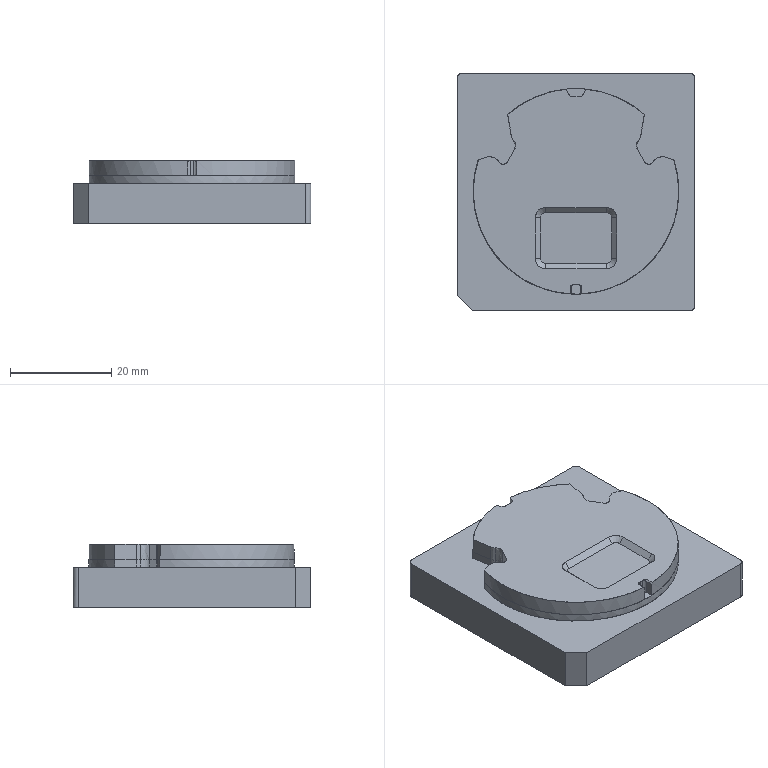NC program | PowerMill | posted with a generic post | part box 47 x 47 x 12.511 mm
Lines 16282 to 17389 of 232111:
N16379 M6
N16380 S8500 M03
N16381 G00 G90 X0.0 Y0.0
N16382 G43 Z11.801 H3
N16383
N16384 G05 P10000 R8
N16385 X-1.9559 Y31.1287
N16386 Z-2.08
N16387 G01 Z-3.28 F360.0
N16388 X-1.5441 Y25.8698 F600.0
N16389 G03 X-1.1674 Y25.6718 I0.4494 J0.3976
N16390 G01 X-0.8465 Y25.6171
N16391 X-0.5643 Y25.5515
N16392 X-0.2822 Y25.4696
N16393 X-0.199 Y25.4403
N16394 G03 X0.199 I0.199 J0.5661
N16395 G01 X0.2822 Y25.4696
N16396 X0.5643 Y25.5515
N16397 X0.8465 Y25.6171
N16398 X1.1287 Y25.6671
N16399 X1.4108 Y25.7015
N16400 X1.693 Y25.7211
N16401 X1.9523 Y25.7257
N16402 G03 X2.2593 Y25.8166 I-0.0106 J0.5999
N16403 G00 Z4.0015
N16404 G01 X7.284 Y30.297 F10000.0
N16405 G00 Z0.9315
N16406 G01 Z-0.2685 F360.0
N16407 X6.0222 Y25.1751 F600.0
N16408 X-18.9848 Y15.2852
N16409 X-18.9833 Y15.0806
N16410 X-18.966 Y14.793
N16411 X-18.9344 Y14.5106
N16412 X-18.9091 Y14.3457
N16413 X-18.5491 Y12.3094
N16414 X-18.8343 Y12.2512
N16415 X-19.2161 Y12.1568
N16416 X-19.495 Y12.0725
N16417 X-19.8583 Y11.9493
N16418 X-21.199 Y11.4604
N16419 X-21.3814 Y11.3897
N16420 X-21.5617 Y11.3136
N16421 X-21.7594 Y11.2206
N16422 X-22.0334 Y11.0742
N16423 X-22.1755 Y10.9915
N16424 X-22.3485 Y10.8815
N16425 X-22.6744 Y10.6481
N16426 X-22.9228 Y10.4449
N16427 X-23.1181 Y10.2662
N16428 X-23.3136 Y10.0694
N16429 X-23.4971 Y9.8645
N16430 X-23.6481 Y9.6794
N16431 X-23.7839 Y9.4976
N16432 X-23.948 Y9.2535
N16433 X-24.0661 Y9.0599
N16434 X-24.1824 Y8.8472
N16435 X-24.2906 Y8.6302
N16436 X-24.4151 Y8.3425
N16437 X-24.5201 Y8.0569
N16438 X12.4545 Y22.6798
N16439 X12.7482 Y22.5176
N16440 X13.3123 Y22.1867
N16441 X14.0252 Y21.7406
N16442 X14.5398 Y21.3978
N16443 X15.0415 Y21.0461
N16444 X15.5786 Y20.6499
N16445 X16.1484 Y20.2049
N16446 X16.5964 Y19.8366
N16447 X17.0379 Y19.4533
N16448 X-25.6557 Y2.5685
N16449 X-25.6952 Y2.1165
N16450 X-25.7221 Y1.7438
N16451 X-25.7538 Y1.1091
N16452 G03 X-25.7718 Y-0.1894 I32.4439 J-1.0979
N16453 G01 X-25.7592 Y-0.7348
N16454 X-25.7264 Y-1.4301
N16455 X-25.6889 Y-1.9481
N16456 X-25.6423 Y-2.4653
N16457 X18.9842 Y15.1839
N16458 X18.9835 Y15.0859
N16459 G02 X18.9091 Y14.3457 I-5.9029 J0.2194
N16460 G01 X18.549 Y12.3091
N16461 X18.75 Y12.2698
N16462 X19.2161 Y12.1568
N16463 X19.4948 Y12.0726
N16464 X19.8555 Y11.9502
N16465 X21.1965 Y11.4614
N16466 X21.3786 Y11.3908
N16467 X21.5624 Y11.3135
N16468 X21.7342 Y11.2323
N16469 X-24.7296 Y-7.1435
N16470 X-24.5357 Y-7.7749
N16471 X-24.279 Y-8.5315
N16472 X-24.0808 Y-9.07
N16473 X-23.8388 Y-9.6817
N16474 X-23.5679 Y-10.3164
N16475 X-23.293 Y-10.9154
N16476 X-23.0058 Y-11.501
N16477 X24.7274 Y7.3769
N16478 X24.7977 Y7.1419
N16479 X24.9346 Y6.6395
N16480 X25.0763 Y6.0727
N16481 X25.2312 Y5.3792
N16482 X25.3226 Y4.9198
N16483 X25.3803 Y4.602
N16484 X25.4836 Y3.9679
N16485 X25.5726 Y3.3334
N16486 X25.6438 Y2.7001
N16487 X-20.473 Y-15.5385
N16488 X-20.1109 Y-16.0027
N16489 X-19.8166 Y-16.361
N16490 X-19.5181 Y-16.7156
N16491 X-19.2019 Y-17.0755
N16492 X-19.0013 Y-17.2971
N16493 X-18.7087 Y-17.6101
N16494 X-18.2485 Y-18.0837
N16495 X-17.8897 Y-18.4363
N16496 X-17.5949 Y-18.7165
N16497 X-17.2957 Y-18.9919
N16498 X-17.0377 Y-19.219
N16499 X25.6558 Y-2.3343
N16500 X25.5832 Y-3.0141
N16501 X25.4974 Y-3.6491
N16502 X25.3955 Y-4.2838
N16503 X25.2768 Y-4.9186
N16504 X25.1764 Y-5.3914
N16505 X25.0694 Y-5.8627
N16506 X24.9355 Y-6.403
N16507 X24.7306 Y-7.1402
N16508 X24.5177 Y-7.8236
N16509 X-12.4535 Y-22.4452
N16510 X-12.2179 Y-22.5761
N16511 X-11.6955 Y-22.8502
N16512 X-11.0463 Y-23.169
N16513 X-10.5089 Y-23.4172
N16514 X-9.9513 Y-23.6579
N16515 X-9.3471 Y-23.9017
N16516 X-8.9157 Y-24.0648
N16517 X-8.3099 Y-24.2802
N16518 X-7.775 Y-24.4554
N16519 X-7.3136 Y-24.5975
N16520 X-6.8223 Y-24.7369
N16521 X-6.0249 Y-24.942
N16522 X21.5338 Y-14.0429
N16523 G00 Z11.801
N16524 G05 P0
N16525 (---------------)
N16526 ( END TOOLPATH : 精公基准台01-平坦面平行-D10 )
N16527 (---------------)
N16528 ( START TOOLPATH : 精公基准台01-基准面偏置-D10 )
N16529 (---------------)
N16530 G00 X0.0 Y0.0 Z9.8015
N16531 G05 P10000 R8
N16532 X-0.6019 Y34.255
N16533 Z-3.51
N16534 G01 Z-4.71 F360.0
N16535 Y28.98 F600.0
N16536 X-0.5663 Y25.8112
N16537 X0.0 Y25.8175
N16538 X0.5663 Y25.8112
N16539 G02 X2.2654 Y25.7174 I-0.551 J-25.4305
N16540 G01 X2.8317 Y25.661
N16541 X3.3981 Y25.5919
N16542 X4.1157 Y25.4857
N16543 X4.5308 Y25.4152
N16544 X5.0971 Y25.307
N16545 X5.6635 Y25.1856
N16546 X6.2298 Y25.051
N16547 X6.7962 Y24.9027
N16548 X7.3625 Y24.7404
N16549 X7.9289 Y24.564
N16550 X8.4952 Y24.3729
N16551 X9.0616 Y24.1671
N16552 X9.6279 Y23.9459
N16553 X10.1943 Y23.7092
N16554 X10.7606 Y23.4562
N16555 X11.327 Y23.1868
N16556 X11.8933 Y22.9
N16557 X12.4597 Y22.5953
N16558 X13.026 Y22.2718
N16559 X13.5924 Y21.9288
N16560 X14.2256 Y21.5212
N16561 X14.7251 Y21.1808
N16562 X15.2914 Y20.7735
N16563 X15.8578 Y20.3418
N16564 X16.499 Y19.8222
N16565 X17.1525 Y19.2558
N16566 X17.3869 Y19.0298
N16567 X17.5568 Y18.8471
N16568 X17.6915 Y18.6895
N16569 X17.9089 Y18.4063
N16570 X18.0723 Y18.1622
N16571 X22.1193 Y20.7449
N16572 G03 X20.6796 Y22.5214 I-8.5455 J-5.4534
N16573 G01 X20.0339 Y23.1489
N16574 G02 X20.4552 Y24.1693 I0.413 J0.4266
N16575 G01 X21.6227 Y24.1529
N16576 G02 X24.1544 Y21.597 I-0.0359 J-2.5674
N16577 G01 X24.1687 Y18.3761
N16578 G02 X23.2908 Y18.2225 I-0.452 J-0.002
N16579 G01 X23.1242 Y18.6908
N16580 G03 X22.1193 Y20.7449 I-9.5502 J-3.3993
N16581 G01 X18.0723 Y18.1622
N16582 X18.1231 Y18.0833
N16583 X18.2901 Y17.7907
N16584 X18.4066 Y17.5568
N16585 X18.5297 Y17.2736
N16586 X18.6339 Y16.9904
N16587 X18.6895 Y16.8151
N16588 X18.7907 Y16.4241
N16589 X18.8448 Y16.1409
N16590 X18.8833 Y15.8578
N16591 X18.9067 Y15.5746
N16592 X18.9151 Y15.2914
N16593 X18.9088 Y15.0082
N16594 X18.8872 Y14.7251
N16595 X18.8507 Y14.4419
N16596 X18.6281 Y13.1786
N16597 G03 X19.3043 Y12.0532 I0.9847 J-0.1742
N16598 G01 X19.7973 Y11.8933
N16599 X21.3431 Y11.327
N16600 X21.5212 Y11.2523
N16601 X21.8044 Y11.1174
N16602 X22.0876 Y10.9608
N16603 X22.4003 Y10.7606
N16604 X22.6539 Y10.5748
N16605 X22.851 Y10.4138
N16606 X23.0914 Y10.1943
N16607 X23.2203 Y10.0651
N16608 X23.4385 Y9.8247
N16609 X23.5986 Y9.6279
N16610 X23.7866 Y9.3699
N16611 X23.9827 Y9.0616
N16612 X24.1381 Y8.7784
N16613 X24.2725 Y8.4952
N16614 X24.353 Y8.3019
N16615 X24.4843 Y7.9289
N16616 X24.658 Y7.3625
N16617 X24.8176 Y6.7962
N16618 X24.963 Y6.2298
N16619 X25.0949 Y5.6635
N16620 X25.2133 Y5.0971
N16621 X25.3184 Y4.5308
N16622 X25.4107 Y3.9644
N16623 X25.4901 Y3.3981
N16624 X25.5567 Y2.8317
N16625 X25.6107 Y2.2654
N16626 X25.6519 Y1.699
N16627 X25.6804 Y1.1327
N16628 X25.6961 Y0.5663
N16629 X25.7003 Y0.0
N16630 X25.6914 Y-0.5663
N16631 X25.6701 Y-1.1327
N16632 X25.6361 Y-1.699
N16633 X25.5899 Y-2.2654
N16634 X25.5307 Y-2.8317
N16635 X25.4588 Y-3.3981
N16636 X25.3742 Y-3.9644
N16637 X25.2766 Y-4.5308
N16638 X25.166 Y-5.0971
N16639 X25.0418 Y-5.6635
N16640 X24.9044 Y-6.2298
N16641 X24.7528 Y-6.7962
N16642 X24.5878 Y-7.3625
N16643 X24.4086 Y-7.9289
N16644 X24.2144 Y-8.4952
N16645 X24.0056 Y-9.0616
N16646 X23.7814 Y-9.6279
N16647 X23.5413 Y-10.1943
N16648 X23.2203 Y-10.8981
N16649 X23.012 Y-11.327
N16650 X22.6539 Y-12.0202
N16651 X22.4131 Y-12.4597
N16652 X22.0856 Y-13.026
N16653 X21.7386 Y-13.5924
N16654 X21.3708 Y-14.1587
N16655 X20.9814 Y-14.7251
N16656 X20.5691 Y-15.2914
N16657 X20.3528 Y-15.5762
N16658 X20.1322 Y-15.8578
N16659 X19.6695 Y-16.4241
N16660 X19.1792 Y-16.9904
N16661 X18.6588 Y-17.5568
N16662 X18.1181 Y-18.1105
N16663 X21.5033 Y-21.5156
N16664 G03 X22.6448 Y-20.3166 I-21.2378 J21.3626
N16665 G01 X23.1332 Y-19.7746
N16666 G02 X24.1738 Y-20.1988 I0.4438 J-0.3998
N16667 G01 X24.1004 Y-21.9892
N16668 G02 X23.5434 Y-23.2871 I-1.98 J0.0812
N16669 G01 X23.3092 Y-23.5288
N16670 G02 X21.9107 Y-24.1365 I-1.4362 J1.3919
N16671 G01 X20.1605 Y-24.1695
N16672 G02 X19.7548 Y-23.1334 I-0.0112 J0.5931
N16673 G01 X20.2976 Y-22.6501
N16674 G03 X21.5033 Y-21.5156 I-20.0312 J22.4962
N16675 G01 X18.1181 Y-18.1105
N16676 X17.8196 Y-18.4025
N16677 X17.5164 Y-18.6895
N16678 X16.8873 Y-19.2558
N16679 X16.4241 Y-19.6505
N16680 X15.8578 Y-20.1079
N16681 X15.2914 Y-20.5392
N16682 X14.7251 Y-20.9469
N16683 X14.1587 Y-21.3315
N16684 X13.5924 Y-21.6949
N16685 X12.9408 Y-22.0876
N16686 X12.4597 Y-22.3611
N16687 X11.9163 Y-22.6539
N16688 X11.327 Y-22.9529
N16689 X10.7606 Y-23.2222
N16690 X10.1943 Y-23.4752
N16691 X9.6279 Y-23.712
N16692 X9.0616 Y-23.9329
N16693 X8.4952 Y-24.1389
N16694 X7.8567 Y-24.353
N16695 X7.3625 Y-24.5062
N16696 X6.7962 Y-24.6685
N16697 X6.2298 Y-24.817
N16698 X5.6635 Y-24.9517
N16699 X5.0971 Y-25.0728
N16700 X4.5308 Y-25.1809
N16701 X3.9644 Y-25.2758
N16702 X3.3981 Y-25.3576
N16703 X2.8317 Y-25.4268
N16704 X2.2654 Y-25.4835
N16705 X1.699 Y-25.5272
N16706 G02 X0.5663 Y-25.5772 I-1.7076 J25.8038
N16707 G01 X0.0 Y-25.5836
N16708 X-0.5663 Y-25.5772
N16709 G02 X-1.699 Y-25.5272 I0.5774 J25.9095
N16710 G01 X-2.2654 Y-25.4835
N16711 X-2.8317 Y-25.4268
N16712 X-3.3981 Y-25.3579
N16713 X-3.9644 Y-25.2758
N16714 X-4.5308 Y-25.1809
N16715 X-5.0971 Y-25.0728
N16716 X-5.6635 Y-24.9517
N16717 X-6.2298 Y-24.817
N16718 X-6.7962 Y-24.6685
N16719 X-7.3625 Y-24.5062
N16720 X-7.9289 Y-24.3297
N16721 X-8.4952 Y-24.1389
N16722 X-9.0616 Y-23.9329
N16723 X-9.6279 Y-23.712
N16724 X-10.1943 Y-23.4752
N16725 X-10.7645 Y-23.2203
N16726 X-11.327 Y-22.9529
N16727 X-11.9163 Y-22.6539
N16728 X-12.4597 Y-22.3614
N16729 X-13.026 Y-22.0378
N16730 X-13.5924 Y-21.6949
N16731 X-14.1587 Y-21.3315
N16732 X-14.7251 Y-20.9469
N16733 X-15.2914 Y-20.5392
N16734 X-15.8578 Y-20.1079
N16735 X-16.4241 Y-19.6507
N16736 X-16.9904 Y-19.166
N16737 X-17.5164 Y-18.6895
N16738 X-17.8181 Y-18.4039
N16739 X-18.1152 Y-18.1136
N16740 X-21.4997 Y-21.5192
N16741 G03 X-20.2974 Y-22.6503 I21.2394 J21.3721
N16742 G01 X-19.7552 Y-23.1331
N16743 G02 X-20.4915 Y-24.0577 I-0.3936 J-0.442
N16744 G01 X-21.3792 Y-23.4273
N16745 G02 X-21.6989 Y-23.1444 I1.1581 J1.6308
N16746 G01 X-23.3258 Y-21.3608
N16747 X-24.0117 Y-20.5681
N16748 G02 X-23.1244 Y-19.7848 I0.4478 J0.387
N16749 G01 X-22.6383 Y-20.3239
N16750 G03 X-21.4997 Y-21.5192 I22.3766 J20.1752
N16751 G01 X-18.1152 Y-18.1136
N16752 X-18.6588 Y-17.5568
N16753 X-19.2558 Y-16.9044
N16754 X-19.6698 Y-16.4241
N16755 X-20.1325 Y-15.8578
N16756 X-20.3529 Y-15.5762
N16757 X-20.5691 Y-15.2914
N16758 X-20.9817 Y-14.7251
N16759 X-21.3711 Y-14.1587
N16760 X-21.7386 Y-13.5924
N16761 X-22.0856 Y-13.026
N16762 X-22.4131 Y-12.4597
N16763 X-22.7214 Y-11.8933
N16764 X-23.012 Y-11.327
N16765 X-23.285 Y-10.7606
N16766 X-23.5413 Y-10.1943
N16767 X-23.7814 Y-9.6279
N16768 X-24.0056 Y-9.0616
N16769 X-24.2144 Y-8.4952
N16770 X-24.4086 Y-7.9289
N16771 X-24.588 Y-7.3625
N16772 X-24.7531 Y-6.7962
N16773 X-24.9044 Y-6.2298
N16774 X-25.0421 Y-5.6635
N16775 X-25.166 Y-5.0971
N16776 X-25.2766 Y-4.5308
N16777 X-25.3742 Y-3.9644
N16778 X-25.4588 Y-3.3981
N16779 X-25.5307 Y-2.8317
N16780 X-25.5899 Y-2.2654
N16781 X-25.6361 Y-1.699
N16782 X-25.6701 Y-1.1327
N16783 X-25.6914 Y-0.5663
N16784 X-25.7003 Y0.0
N16785 X-25.6961 Y0.5663
N16786 X-25.6804 Y1.1327
N16787 X-25.6519 Y1.699
N16788 X-25.6101 Y2.2654
N16789 X-25.5567 Y2.8317
N16790 X-25.4857 Y3.4321
N16791 X-25.411 Y3.9644
N16792 X-25.3181 Y4.5308
N16793 X-25.2133 Y5.0971
N16794 X-25.0949 Y5.6635
N16795 X-24.963 Y6.2298
N16796 X-24.8176 Y6.7962
N16797 X-24.658 Y7.3625
N16798 X-24.4843 Y7.9289
N16799 X-24.353 Y8.3019
N16800 X-24.2725 Y8.4952
N16801 X-24.1382 Y8.7784
N16802 X-23.9827 Y9.0616
N16803 X-23.7866 Y9.3699
N16804 X-23.5986 Y9.6279
N16805 X-23.4197 Y9.8465
N16806 X-23.2203 Y10.0651
N16807 X-23.0914 Y10.1943
N16808 X-22.8727 Y10.3951
N16809 X-22.6539 Y10.5748
N16810 X-22.4003 Y10.7606
N16811 X-22.0876 Y10.9608
N16812 X-21.8044 Y11.1174
N16813 X-21.5212 Y11.2523
N16814 X-21.3431 Y11.327
N16815 X-19.7973 Y11.8933
N16816 X-19.3043 Y12.0532
N16817 G03 X-18.6281 Y13.1786 I-0.3085 J0.9512
N16818 G01 X-18.8506 Y14.4419
N16819 X-18.8872 Y14.7251
N16820 X-18.9085 Y15.0082
N16821 X-18.9151 Y15.2914
N16822 X-18.9066 Y15.5746
N16823 X-18.8833 Y15.8578
N16824 X-18.8448 Y16.1409
N16825 X-18.7907 Y16.4241
N16826 X-18.6895 Y16.8151
N16827 X-18.6339 Y16.9904
N16828 X-18.5296 Y17.2736
N16829 X-18.4066 Y17.5568
N16830 X-18.2743 Y17.8201
N16831 X-18.0985 Y18.1231
N16832 X-17.9713 Y18.3131
N16833 X-21.9629 Y20.9979
N16834 G03 X-23.1223 Y18.7037 I8.6103 J-5.7915
N16835 G01 X-23.2901 Y18.235
N16836 G02 X-24.1685 Y18.3896 I-0.426 J0.1524
N16837 G01 X-24.1531 Y21.5997
N16838 G02 X-21.6204 Y24.1538 I2.5667 J-0.0124
N16839 G01 X-20.4578 Y24.1692
N16840 G02 X-20.0544 Y23.1344 I0.0078 J-0.5931
N16841 G01 X-20.2751 Y22.9367
N16842 G03 X-21.9629 Y20.9979 I6.9226 J-7.7303
N16843 G01 X-17.9713 Y18.3131
N16844 X-17.9089 Y18.4063
N16845 X-17.6915 Y18.6895
N16846 X-17.5568 Y18.8471
N16847 X-17.3869 Y19.0298
N16848 X-17.1525 Y19.2558
N16849 X-16.499 Y19.8222
N16850 X-15.798 Y20.3885
N16851 X-15.2914 Y20.7735
N16852 X-14.7251 Y21.1808
N16853 X-14.1587 Y21.5658
N16854 X-13.5924 Y21.9291
N16855 X-13.026 Y22.2718
N16856 X-12.3532 Y22.6539
N16857 X-11.8933 Y22.9
N16858 X-11.2581 Y23.2203
N16859 X-10.7606 Y23.4562
N16860 X-10.1943 Y23.7092
N16861 X-9.6279 Y23.9459
N16862 X-9.0616 Y24.1671
N16863 X-8.4952 Y24.3729
N16864 X-7.9289 Y24.564
N16865 X-7.3625 Y24.7404
N16866 X-6.7962 Y24.9027
N16867 X-6.2298 Y25.051
N16868 X-5.6635 Y25.1856
N16869 X-5.0971 Y25.307
N16870 X-4.5308 Y25.4149
N16871 X-3.9644 Y25.51
N16872 X-3.3981 Y25.5919
N16873 X-2.8317 Y25.661
N16874 X-2.2654 Y25.7174
N16875 G02 X-0.5663 Y25.8112 I2.2499 J-25.3333
N16876 G01 X-0.6019 Y28.98
N16877 G00 Z9.8015
N16878 G05 P0
N16879 (---------------)
N16880 ( END TOOLPATH : 精公基准台01-基准面偏置-D10 )
N16881 (---------------)
N16882 ( START TOOLPATH : 精公基准台01-外形侧光-D10 )
N16883 (---------------)
N16884 G00 X0.0 Y0.0 Z10.801
N16885 G05 P10000 R8
N16886 X18.9615 Y-17.3661
N16887 Z-3.48
N16888 G01 Z-4.68 F360.0
N16889 G03 X17.9006 Y-17.8048 I-0.0009 J-1.5 F600.0
N16890 G02 X0.0115 Y-25.2132 I-17.9006 J17.9219
N16891 G02 X-24.742 Y-5.3107 I-0.0115 J25.3303
N16892 G02 X-24.1127 Y7.8761 I24.7432 J5.4277
N16893 G02 X-21.0885 Y11.0285 I4.7658 J-1.5451
N16894 G01 X-19.5823 Y11.5771
N16895 G02 X-18.2613 Y11.9071 I2.4706 J-7.082
N16896 G03 X-18.0726 Y12.1636 I-0.0279 J0.2182
N16897 G01 X-18.2711 Y13.2858
N16898 X-18.4699 Y14.4096
N16899 G02 X-16.848 Y19.0318 I4.935 J0.864
N16900 G02 X16.8496 Y19.0304 I16.848 J-18.9146
N16901 G02 X18.4697 Y14.408 I-3.3146 J-3.7568
N16902 G01 X18.0726 Y12.1636
N16903 G03 X18.2608 Y11.9072 I0.2166 J-0.0383
N16904 G02 X19.5605 Y11.5846 I-1.1507 J-7.4174
N16905 G02 X21.0899 Y11.028 I-50.0728 J-139.9594
N16906 G02 X24.1135 Y7.8738 I-1.743 J-4.6971
N16907 G02 X17.9006 Y-17.8048 I-24.1135 J-7.7567
N16908 G03 X17.4606 Y-18.8652 I1.06 J-1.0613
N16909 G01 X18.9048 Y-17.3097
N16910 G03 X17.8438 Y-17.7484 I-0.001 J-1.5
N16911 G02 X0.0115 Y-25.1332 I-17.8438 J17.8655
N16912 G02 X-24.6637 Y-5.2941 I-0.0115 J25.2503
N16913 G02 X-24.0371 Y7.8499 I24.6654 J5.4111
N16914 G02 X-21.0611 Y10.9534 I4.6901 J-1.5189
N16915 G01 X-19.5576 Y11.501
N16916 G02 X-18.2512 Y11.8277 I2.4472 J-7.011
N16917 G03 X-17.9938 Y12.1776 I-0.038 J0.2976
N16918 G01 X-18.1924 Y13.2998
N16919 X-18.3909 Y14.4219
N16920 G02 X-16.7952 Y18.9717 I4.8559 J0.8517
N16921 G02 X16.7952 I16.7952 J-18.8545
N16922 G02 X18.3909 Y14.4219 I-3.2602 J-3.6981
N16923 G01 X17.9938 Y12.1776
N16924 G03 X18.2504 Y11.8278 I0.2954 J-0.0523
N16925 G02 X19.5335 Y11.5093 I-1.1406 J-7.339
N16926 G02 X21.0611 Y10.9534 I-50.0448 J-139.8831
N16927 G02 X24.0371 Y7.8499 I-1.7141 J-4.6224
N16928 G02 X17.8438 Y-17.7484 I-24.0371 J-7.7328
N16929 G03 X17.4038 Y-18.8088 I1.0601 J-1.0613
N16930 G00 Z10.801
N16931 G05 P0
N16932 (---------------)
N16933 ( END TOOLPATH : 精公基准台01-外形侧光-D10 )
N16934 (---------------)
N16935 ( START TOOLPATH : 精公基准台01-基准台侧光-D10 )
N16936 (---------------)
N16937 G00 X0.0 Y0.0 Z9.8015
N16938 G05 P10000 R8
N16939 X28.8261 Y-31.5925
N16940 Z-11.41
N16941 G01 Z-12.61 F360.0
N16942 G03 X25.9747 Y-27.4852 I-1.4257 J2.0536 F600.0
N16943 G01 X25.8115 Y-27.5986
N16944 X25.8098 Y-27.5997
N16945 X25.8081 Y-27.6008
N16946 X25.5992 Y-27.7307
N16947 X25.5982 Y-27.7313
N16948 X25.5971 Y-27.732
N16949 X25.4898 Y-27.7941
N16950 X25.4884 Y-27.7948
N16951 X25.487 Y-27.7956
N16952 X25.1708 Y-27.9619
N16953 X25.1687 Y-27.963
N16954 X25.1666 Y-27.964
N16955 X24.8505 Y-28.1073
N16956 X24.8484 Y-28.1082
N16957 X24.8462 Y-28.109
N16958 X24.5301 Y-28.231
N16959 X24.528 Y-28.2318
N16960 X24.5259 Y-28.2325
N16961 X24.2097 Y-28.3346
N16962 X24.2082 Y-28.3351
N16963 X24.2067 Y-28.3355
N16964 X24.0765 Y-28.3721
N16965 X24.0754 Y-28.3724
N16966 X24.0743 Y-28.3726
N16967 X23.8885 Y-28.4193
N16968 X23.8867 Y-28.4197
N16969 X23.885 Y-28.4201
N16970 X23.5688 Y-28.4846
N16971 X23.5669 Y-28.485
N16972 X23.5649 Y-28.4853
N16973 X23.2488 Y-28.5337
N16974 X23.2465 Y-28.534
N16975 X23.2443 Y-28.5342
N16976 X22.9281 Y-28.5642
N16977 X22.9262 Y-28.5644
N16978 X22.9242 Y-28.5645
N16979 X22.608 Y-28.5788
N16980 X22.6064 Y-28.5789
N16981 X22.6047
N16982 X22.2885 Y-28.58
N16983 X22.2884
N16984 X22.2883
N16985 X-20.3914
N16986 X-20.3919
N16987 X-20.3925
N16988 X-20.7086 Y-28.5757
N16989 X-20.711 Y-28.5756
N16990 X-20.7134 Y-28.5755
N16991 X-21.0295 Y-28.5523
N16992 X-21.0321 Y-28.5521
N16993 X-21.0346 Y-28.5518
N16994 X-21.3507 Y-28.5082
N16995 X-21.3533 Y-28.5078
N16996 X-21.3558 Y-28.5074
N16997 X-21.672 Y-28.4429
N16998 X-21.6743 Y-28.4424
N16999 X-21.6766 Y-28.4419
N17000 X-21.9375 Y-28.3723
N17001 X-21.9401 Y-28.3716
N17002 X-21.9426 Y-28.3708
N17003 X-22.3139 Y-28.2451
N17004 X-22.3167 Y-28.2441
N17005 X-22.3194 Y-28.243
N17006 X-22.6356 Y-28.1093
N17007 X-22.6373 Y-28.1085
N17008 X-22.639 Y-28.1077
N17009 X-22.7571 Y-28.051
N17010 X-22.7584 Y-28.0504
N17011 X-22.7597 Y-28.0497
N17012 X-22.9577 Y-27.9459
N17013 X-22.9598 Y-27.9448
N17014 X-22.9618 Y-27.9436
N17015 X-23.278 Y-27.7531
N17016 X-23.2806 Y-27.7515
N17017 X-23.2831 Y-27.7498
N17018 X-23.5992 Y-27.525
N17019 X-23.601 Y-27.5237
N17020 X-23.6028 Y-27.5223
N17021 X-23.7443 Y-27.4091
N17022 X-23.7456 Y-27.408
N17023 X-23.7469 Y-27.4069
N17024 X-23.9215 Y-27.2549
N17025 X-23.9229 Y-27.2537
N17026 X-23.9243 Y-27.2524
N17027 X-24.0959 Y-27.0883
N17028 X-24.0966 Y-27.0877
N17029 X-24.0972 Y-27.087
N17030 X-27.087 Y-24.0972
N17031 X-27.0877 Y-24.0966
N17032 X-27.0883 Y-24.0959
N17033 X-27.2524 Y-23.9243
N17034 X-27.2537 Y-23.9229
N17035 X-27.2549 Y-23.9215
N17036 X-27.4069 Y-23.7469
N17037 X-27.408 Y-23.7456
N17038 X-27.4091 Y-23.7443
N17039 X-27.5223 Y-23.6028
N17040 X-27.5236 Y-23.6012
N17041 X-27.5248 Y-23.5995
N17042 X-27.7278 Y-23.3164
N17043 X-27.7295 Y-23.3139
N17044 X-27.7311 Y-23.3113
N17045 X-27.9434 Y-22.9621
N17046 X-27.9447 Y-22.9599
N17047 X-27.9459 Y-22.9577
N17048 X-28.0497 Y-22.7597
N17049 X-28.0504 Y-22.7584
N17050 X-28.051 Y-22.7571
N17051 X-28.1077 Y-22.639
N17052 X-28.1085 Y-22.6373
N17053 X-28.1093 Y-22.6356
N17054 X-28.243 Y-22.3194
N17055 X-28.244 Y-22.3169
N17056 X-28.2449 Y-22.3144
N17057 X-28.354 Y-21.9982
N17058 X-28.3548 Y-21.9957
N17059 X-28.3556 Y-21.9932
N17060 X-28.4417 Y-21.677
N17061 X-28.4424 Y-21.6745
N17062 X-28.4429 Y-21.672
N17063 X-28.5074 Y-21.3558
N17064 X-28.5078 Y-21.3533
N17065 X-28.5082 Y-21.3507
N17066 X-28.5518 Y-21.0346
N17067 X-28.5521 Y-21.0321
N17068 X-28.5523 Y-21.0295
N17069 X-28.5755 Y-20.7134
N17070 X-28.5756 Y-20.711
N17071 X-28.5757 Y-20.7086
N17072 X-28.58 Y-20.3925
N17073 Y-20.3919
N17074 Y-20.3914
N17075 Y22.2883
N17076 Y22.2884
N17077 Y22.2885
N17078 X-28.5789 Y22.6047
N17079 Y22.6063
N17080 X-28.5788 Y22.6079
N17081 X-28.5652 Y22.924
N17082 X-28.565 Y22.9262
N17083 X-28.5649 Y22.9283
N17084 X-28.5342 Y23.2444
N17085 X-28.534 Y23.2465
N17086 X-28.5337 Y23.2486
N17087 X-28.486 Y23.5648
N17088 X-28.4857 Y23.5669
N17089 X-28.4853 Y23.569
N17090 X-28.4201 Y23.8852
N17091 X-28.4196 Y23.8873
N17092 X-28.4191 Y23.8894
N17093 X-28.3358 Y24.2055
N17094 X-28.3352 Y24.2077
N17095 X-28.3346 Y24.2098
N17096 X-28.2323 Y24.5259
N17097 X-28.2316 Y24.528
N17098 X-28.2308 Y24.53
N17099 X-28.109 Y24.8462
N17100 X-28.1084 Y24.8477
N17101 X-28.1078 Y24.8492
N17102 X-28.0523 Y24.9775
N17103 X-28.0518 Y24.9786
N17104 X-28.0513 Y24.9797
N17105 X-27.9633 Y25.1675
N17106 X-27.9625 Y25.1692
N17107 X-27.9617 Y25.1708
N17108 X-27.7956 Y25.4869
N17109 X-27.7949 Y25.4884
N17110 X-27.7941 Y25.4898
N17111 X-27.732 Y25.5971
N17112 X-27.7314 Y25.5981
N17113 X-27.7307 Y25.5992
N17114 X-27.6012 Y25.808
N17115 X-27.6001 Y25.8096
N17116 X-27.5991 Y25.8112
N17117 X-27.4125 Y26.0824
N17118 X-27.411 Y26.0845
N17119 X-27.4094 Y26.0866
N17120 X-27.1239 Y26.4478
N17121 X-27.122 Y26.4501
N17122 X-27.12 Y26.4523
N17123 X-26.8297 Y26.7684
N17124 X-26.8285 Y26.7697
N17125 X-26.8273 Y26.7709
N17126 X-26.7709 Y26.8273
N17127 X-26.7698 Y26.8284
N17128 X-26.7686 Y26.8295
N17129 X-26.4878 Y27.0892
N17130 X-26.4858 Y27.091
N17131 X-26.4837 Y27.0928
N17132 X-26.1322 Y27.3757
N17133 X-26.1299 Y27.3774
N17134 X-26.1276 Y27.3791
N17135 X-25.8115 Y27.5986
N17136 X-25.8098 Y27.5997
N17137 X-25.8081 Y27.6008
N17138 X-25.5992 Y27.7307
N17139 X-25.5982 Y27.7313
N17140 X-25.5971 Y27.732
N17141 X-25.4898 Y27.7941
N17142 X-25.4884 Y27.7948
N17143 X-25.487 Y27.7956
N17144 X-25.1708 Y27.9619
N17145 X-25.1687 Y27.963
N17146 X-25.1666 Y27.964
N17147 X-24.8505 Y28.1073
N17148 X-24.8484 Y28.1082
N17149 X-24.8462 Y28.109
N17150 X-24.5301 Y28.231
N17151 X-24.528 Y28.2318
N17152 X-24.5259 Y28.2325
N17153 X-24.2097 Y28.3346
N17154 X-24.2076 Y28.3353
N17155 X-24.2055 Y28.3359
N17156 X-23.8894 Y28.4191
N17157 X-23.8872 Y28.4197
N17158 X-23.885 Y28.4201
N17159 X-23.5688 Y28.4846
N17160 X-23.5669 Y28.485
N17161 X-23.5649 Y28.4853
N17162 X-23.2488 Y28.5337
N17163 X-23.2465 Y28.534
N17164 X-23.2443 Y28.5342
N17165 X-22.9281 Y28.5642
N17166 X-22.9262 Y28.5644
N17167 X-22.9242 Y28.5645
N17168 X-22.608 Y28.5788
N17169 X-22.6064 Y28.5789
N17170 X-22.6047
N17171 X-22.2885 Y28.58
N17172 X-22.2884
N17173 X-22.2883
N17174 X22.2883
N17175 X22.2884
N17176 X22.2885
N17177 X22.6047 Y28.5789
N17178 X22.6063
N17179 X22.6079 Y28.5788
N17180 X22.924 Y28.5652
N17181 X22.9262 Y28.565
N17182 X22.9283 Y28.5649
N17183 X23.2444 Y28.5342
N17184 X23.2465 Y28.534
N17185 X23.2486 Y28.5337
N17186 X23.5648 Y28.486
N17187 X23.5669 Y28.4857
N17188 X23.569 Y28.4853
N17189 X23.8852 Y28.4201
N17190 X23.8873 Y28.4196
N17191 X23.8894 Y28.4191
N17192 X24.2055 Y28.3358
N17193 X24.2077 Y28.3352
N17194 X24.2098 Y28.3346
N17195 X24.5259 Y28.2323
N17196 X24.528 Y28.2316
N17197 X24.53 Y28.2308
N17198 X24.8462 Y28.109
N17199 X24.8477 Y28.1084
N17200 X24.8492 Y28.1078
N17201 X24.9775 Y28.0523
N17202 X24.9786 Y28.0518
N17203 X24.9797 Y28.0513
N17204 X25.1675 Y27.9633
N17205 X25.1692 Y27.9625
N17206 X25.1708 Y27.9617
N17207 X25.4869 Y27.7956
N17208 X25.4884 Y27.7949
N17209 X25.4898 Y27.7941
N17210 X25.5971 Y27.732
N17211 X25.5981 Y27.7314
N17212 X25.5992 Y27.7307
N17213 X25.808 Y27.6012
N17214 X25.8096 Y27.6001
N17215 X25.8112 Y27.5991
N17216 X26.0824 Y27.4125
N17217 X26.0845 Y27.411
N17218 X26.0866 Y27.4094
N17219 X26.4478 Y27.1239
N17220 X26.4501 Y27.122
N17221 X26.4523 Y27.12
N17222 X26.7684 Y26.8297
N17223 X26.7697 Y26.8285
N17224 X26.7709 Y26.8273
N17225 X26.8273 Y26.7709
N17226 X26.8284 Y26.7698
N17227 X26.8295 Y26.7686
N17228 X27.0892 Y26.4878
N17229 X27.091 Y26.4858
N17230 X27.0928 Y26.4837
N17231 X27.3757 Y26.1322
N17232 X27.3774 Y26.1299
N17233 X27.3791 Y26.1276
N17234 X27.5986 Y25.8115
N17235 X27.5997 Y25.8098
N17236 X27.6008 Y25.8081
N17237 X27.7307 Y25.5992
N17238 X27.7313 Y25.5982
N17239 X27.732 Y25.5971
N17240 X27.7941 Y25.4898
N17241 X27.7948 Y25.4884
N17242 X27.7956 Y25.487
N17243 X27.9619 Y25.1708
N17244 X27.963 Y25.1687
N17245 X27.964 Y25.1666
N17246 X28.1073 Y24.8505
N17247 X28.1082 Y24.8484
N17248 X28.109 Y24.8462
N17249 X28.231 Y24.5301
N17250 X28.2318 Y24.528
N17251 X28.2325 Y24.5259
N17252 X28.3346 Y24.2097
N17253 X28.3353 Y24.2076
N17254 X28.3359 Y24.2055
N17255 X28.4191 Y23.8894
N17256 X28.4196 Y23.8872
N17257 X28.4201 Y23.885
N17258 X28.4846 Y23.5688
N17259 X28.485 Y23.5669
N17260 X28.4853 Y23.5649
N17261 X28.5337 Y23.2488
N17262 X28.534 Y23.2465
N17263 X28.5342 Y23.2443
N17264 X28.5642 Y22.9281
N17265 X28.5644 Y22.9262
N17266 X28.5645 Y22.9242
N17267 X28.5788 Y22.608
N17268 X28.5789 Y22.6064
N17269 Y22.6047
N17270 X28.58 Y22.2885
N17271 Y22.2884
N17272 Y22.2883
N17273 Y0.0
N17274 Y-22.2883
N17275 Y-22.2884
N17276 Y-22.2885
N17277 X28.5789 Y-22.6047
N17278 Y-22.6063
N17279 X28.5788 Y-22.6079
N17280 X28.5652 Y-22.924
N17281 X28.565 Y-22.9262
N17282 X28.5649 Y-22.9283
N17283 X28.5342 Y-23.2444
N17284 X28.534 Y-23.2465
N17285 X28.5337 Y-23.2486
N17286 X28.486 Y-23.5648
N17287 X28.4857 Y-23.5669
N17288 X28.4853 Y-23.569
N17289 X28.4201 Y-23.8852
N17290 X28.4196 Y-23.8873
N17291 X28.4191 Y-23.8894
N17292 X28.3358 Y-24.2055
N17293 X28.3352 Y-24.2077
N17294 X28.3346 Y-24.2098
N17295 X28.2323 Y-24.5259
N17296 X28.2316 Y-24.528
N17297 X28.2308 Y-24.53
N17298 X28.109 Y-24.8462
N17299 X28.1084 Y-24.8477
N17300 X28.1078 Y-24.8492
N17301 X28.0523 Y-24.9775
N17302 X28.0518 Y-24.9786
N17303 X28.0513 Y-24.9797
N17304 X27.9633 Y-25.1675
N17305 X27.9625 Y-25.1692
N17306 X27.9617 Y-25.1708
N17307 X27.7956 Y-25.4869
N17308 X27.7949 Y-25.4884
N17309 X27.7941 Y-25.4898
N17310 X27.732 Y-25.5971
N17311 X27.7314 Y-25.5981
N17312 X27.7307 Y-25.5992
N17313 X27.6012 Y-25.808
N17314 X27.6001 Y-25.8096
N17315 X27.5991 Y-25.8112
N17316 X27.4125 Y-26.0824
N17317 X27.411 Y-26.0845
N17318 X27.4094 Y-26.0866
N17319 X27.1239 Y-26.4478
N17320 X27.122 Y-26.4501
N17321 X27.12 Y-26.4523
N17322 X26.8297 Y-26.7684
N17323 X26.8285 Y-26.7697
N17324 X26.8273 Y-26.7709
N17325 X26.7709 Y-26.8273
N17326 X26.7698 Y-26.8284
N17327 X26.7686 Y-26.8295
N17328 X26.4878 Y-27.0892
N17329 X26.4858 Y-27.091
N17330 X26.4837 Y-27.0928
N17331 X26.1322 Y-27.3757
N17332 X26.1299 Y-27.3774
N17333 X26.1276 Y-27.3791
N17334 X25.9747 Y-27.4852
N17335 G03 X28.8261 Y-31.5925 I1.4257 J-2.0537
N17336 G01 X28.7746 Y-31.5308
N17337 G03 X25.9232 Y-27.4236 I-1.4257 J2.0536
N17338 G01 X25.7659 Y-27.5328
N17339 X25.557 Y-27.6627
N17340 X25.4497 Y-27.7248
N17341 X25.1336 Y-27.8911
N17342 X24.8174 Y-28.0344
N17343 X24.5013 Y-28.1564
N17344 X24.1851 Y-28.2585
N17345 X24.0549 Y-28.295
N17346 X23.869 Y-28.3417
N17347 X23.5529 Y-28.4062
N17348 X23.2367 Y-28.4546
N17349 X22.9206 Y-28.4846
N17350 X22.6044 Y-28.4989
N17351 X22.2883 Y-28.5
N17352 X-20.3914
N17353 X-20.7075 Y-28.4957
N17354 X-21.0237 Y-28.4725
N17355 X-21.3398 Y-28.429
N17356 X-21.656 Y-28.3645
N17357 X-21.9169 Y-28.295
N17358 X-22.2883 Y-28.1693
N17359 X-22.6044 Y-28.0356
N17360 X-22.7225 Y-27.9789
N17361 X-22.9206 Y-27.875
N17362 X-23.2367 Y-27.6846
N17363 X-23.5529 Y-27.4598
N17364 X-23.6943 Y-27.3466
N17365 X-23.869 Y-27.1946
N17366 X-24.0406 Y-27.0305
N17367 X-27.0305 Y-24.0406
N17368 X-27.1946 Y-23.869
N17369 X-27.3466 Y-23.6943
N17370 X-27.4598 Y-23.5529
N17371 X-27.6627 Y-23.2698
N17372 X-27.875 Y-22.9206
N17373 X-27.9789 Y-22.7225
N17374 X-28.0356 Y-22.6044
N17375 X-28.1693 Y-22.2883
N17376 X-28.2784 Y-21.9721
N17377 X-28.3645 Y-21.656
N17378 X-28.429 Y-21.3398
N17379 X-28.4725 Y-21.0237
N17380 X-28.4957 Y-20.7075
N17381 X-28.5 Y-20.3914
N17382 Y22.2883
N17383 X-28.4989 Y22.6044
N17384 X-28.4852 Y22.9206
N17385 X-28.4546 Y23.2367
N17386 X-28.4069 Y23.5529
N17387 X-28.3417 Y23.869
N17388 X-28.2584 Y24.1851
N17389 X-28.1562 Y24.5013
N17390 X-28.0344 Y24.8174
N17391 X-27.9789 Y24.9458
N17392 X-27.8909 Y25.1336
N17393 X-27.7248 Y25.4497
N17394 X-27.6627 Y25.557
N17395 X-27.5332 Y25.7659
N17396 X-27.3466 Y26.037
N17397 X-27.0611 Y26.3982
N17398 X-26.7708 Y26.7143
N17399 X-26.7143 Y26.7708
N17400 X-26.4335 Y27.0305
N17401 X-26.082 Y27.3134
N17402 X-25.7659 Y27.5328
N17403 X-25.557 Y27.6627
N17404 X-25.4497 Y27.7248
N17405 X-25.1336 Y27.8911
N17406 X-24.8174 Y28.0344
N17407 X-24.5013 Y28.1564
N17408 X-24.1851 Y28.2585
N17409 X-23.869 Y28.3417
N17410 X-23.5529 Y28.4063
N17411 X-23.2367 Y28.4546
N17412 X-22.9206 Y28.4846
N17413 X-22.6044 Y28.4989
N17414 X-22.2883 Y28.5
N17415 X22.2883
N17416 X22.6044 Y28.4989
N17417 X22.9206 Y28.4852
N17418 X23.2367 Y28.4546
N17419 X23.5529 Y28.4069
N17420 X23.869 Y28.3417
N17421 X24.1851 Y28.2584
N17422 X24.5013 Y28.1562
N17423 X24.8174 Y28.0344
N17424 X24.9458 Y27.9789
N17425 X25.1336 Y27.8909
N17426 X25.4497 Y27.7248
N17427 X25.557 Y27.6627
N17428 X25.7659 Y27.5332
N17429 X26.037 Y27.3466
N17430 X26.3982 Y27.0611
N17431 X26.7143 Y26.7708
N17432 X26.7708 Y26.7143
N17433 X27.0305 Y26.4335
N17434 X27.3134 Y26.082
N17435 X27.5328 Y25.7659
N17436 X27.6627 Y25.557
N17437 X27.7248 Y25.4497
N17438 X27.8911 Y25.1336
N17439 X28.0344 Y24.8174
N17440 X28.1564 Y24.5013
N17441 X28.2585 Y24.1851
N17442 X28.3417 Y23.869
N17443 X28.4062 Y23.5529
N17444 X28.4546 Y23.2367
N17445 X28.4846 Y22.9206
N17446 X28.4989 Y22.6044
N17447 X28.5 Y22.2883
N17448 Y0.0
N17449 Y-22.2883
N17450 X28.4989 Y-22.6044
N17451 X28.4852 Y-22.9206
N17452 X28.4546 Y-23.2367
N17453 X28.4069 Y-23.5529
N17454 X28.3417 Y-23.869
N17455 X28.2584 Y-24.1851
N17456 X28.1562 Y-24.5013
N17457 X28.0344 Y-24.8174
N17458 X27.9789 Y-24.9458
N17459 X27.8909 Y-25.1336
N17460 X27.7248 Y-25.4497
N17461 X27.6627 Y-25.557
N17462 X27.5332 Y-25.7659
N17463 X27.3466 Y-26.037
N17464 X27.0611 Y-26.3982
N17465 X26.7708 Y-26.7143
N17466 X26.7143 Y-26.7708
N17467 X26.4335 Y-27.0305
N17468 X26.082 Y-27.3134
N17469 X25.9232 Y-27.4236
N17470 G03 X28.7747 Y-31.5308 I1.4258 J-2.0536
N17471 G00 Z9.8015
N17472 G05 P0
N17473 (---------------)
N17474 ( END TOOLPATH : 精公基准台01-基准台侧光-D10 )
N17475 (---------------)
N17476
N17477 M05
N17478 G53 Z0.0
N17479 (---------------)
N17480 ( START TOOLPATH : 精公精光01-等高-D4 )
N17481 (---------------)
N17482 ( TOOL NO.    :14 )
N17483 ( TOOL TYPE   : ENDMILL)
N17484 ( TOOL ID     : D4_1_1)
N17485 ( TOOL DIA    : 4.0 LENGTH 59.68)
N17486 T14